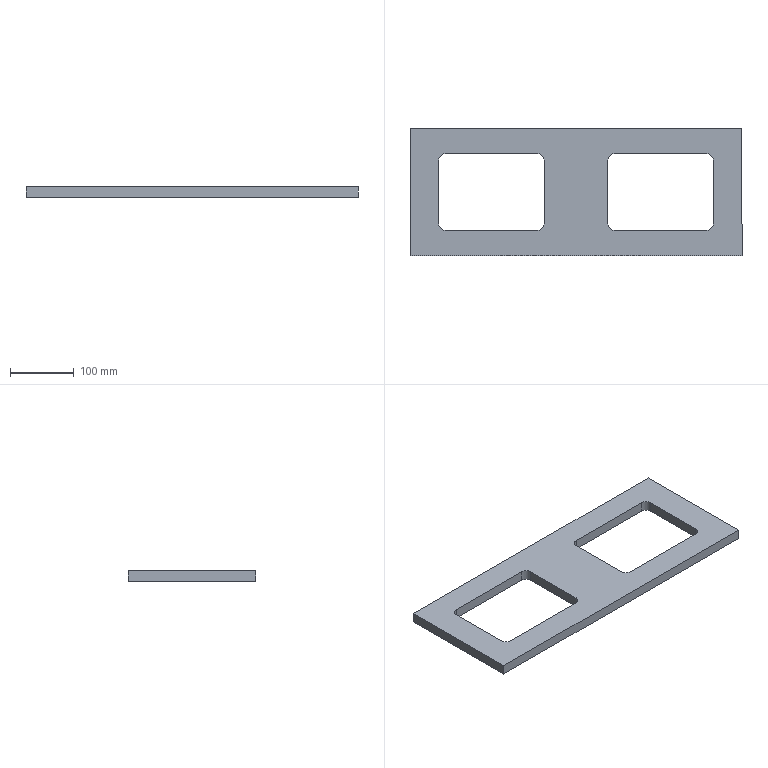Part | SolidWorks | features Extrusion 1 | 1 solid | 22 faces | box 520 x 200 x 16 mm | volume 1033147 mm3 | plane 14 | cylinder 8 | commonest cylinder face diameters 20 x8
STEP:
#1=CARTESIAN_POINT('',(-50.151,129.965,16.));
#2=VERTEX_POINT('',#1);
#3=CARTESIAN_POINT('',(-60.151,119.965,16.));
#4=VERTEX_POINT('',#3);
#5=CARTESIAN_POINT('',(-50.151,119.965,16.));
#6=DIRECTION('',(0.,0.,1.));
#7=DIRECTION('',(-1.,0.,0.));
#8=AXIS2_PLACEMENT_3D('',#5,#6,#7);
#9=CIRCLE('',#8,10.);
#10=EDGE_CURVE('',#2,#4,#9,.T.);
#11=ORIENTED_EDGE('',*,*,#10,.F.);
#12=CARTESIAN_POINT('',(94.849,129.965,16.));
#13=VERTEX_POINT('',#12);
#14=CARTESIAN_POINT('',(94.849,129.965,16.));
#15=DIRECTION('',(-1.,0.,0.));
#16=VECTOR('',#15,1000.);
#17=LINE('',#14,#16);
#18=EDGE_CURVE('',#13,#2,#17,.T.);
#19=ORIENTED_EDGE('',*,*,#18,.F.);
#20=CARTESIAN_POINT('',(104.849,119.965,16.));
#21=VERTEX_POINT('',#20);
#22=CARTESIAN_POINT('',(94.849,119.965,16.));
#23=DIRECTION('',(0.,0.,1.));
#24=DIRECTION('',(-1.,0.,0.));
#25=AXIS2_PLACEMENT_3D('',#22,#23,#24);
#26=CIRCLE('',#25,10.);
#27=EDGE_CURVE('',#21,#13,#26,.T.);
#28=ORIENTED_EDGE('',*,*,#27,.F.);
#29=CARTESIAN_POINT('',(104.849,19.965,16.));
#30=VERTEX_POINT('',#29);
#31=CARTESIAN_POINT('',(104.849,19.965,16.));
#32=DIRECTION('',(0.,1.,0.));
#33=VECTOR('',#32,1000.);
#34=LINE('',#31,#33);
#35=EDGE_CURVE('',#30,#21,#34,.T.);
#36=ORIENTED_EDGE('',*,*,#35,.F.);
#37=CARTESIAN_POINT('',(94.849,9.965,16.));
#38=VERTEX_POINT('',#37);
#39=CARTESIAN_POINT('',(94.849,19.965,16.));
#40=DIRECTION('',(0.,0.,1.));
#41=DIRECTION('',(1.,0.,0.));
#42=AXIS2_PLACEMENT_3D('',#39,#40,#41);
#43=CIRCLE('',#42,10.);
#44=EDGE_CURVE('',#38,#30,#43,.T.);
#45=ORIENTED_EDGE('',*,*,#44,.F.);
#46=CARTESIAN_POINT('',(-50.151,9.965,16.));
#47=VERTEX_POINT('',#46);
#48=CARTESIAN_POINT('',(-50.151,9.965,16.));
#49=DIRECTION('',(1.,0.,0.));
#50=VECTOR('',#49,1000.);
#51=LINE('',#48,#50);
#52=EDGE_CURVE('',#47,#38,#51,.T.);
#53=ORIENTED_EDGE('',*,*,#52,.F.);
#54=CARTESIAN_POINT('',(-60.151,19.965,16.));
#55=VERTEX_POINT('',#54);
#56=CARTESIAN_POINT('',(-50.151,19.965,16.));
#57=DIRECTION('',(0.,0.,1.));
#58=DIRECTION('',(-1.,0.,0.));
#59=AXIS2_PLACEMENT_3D('',#56,#57,#58);
#60=CIRCLE('',#59,10.);
#61=EDGE_CURVE('',#55,#47,#60,.T.);
#62=ORIENTED_EDGE('',*,*,#61,.F.);
#63=CARTESIAN_POINT('',(-60.151,119.965,16.));
#64=DIRECTION('',(0.,-1.,0.));
#65=VECTOR('',#64,1000.);
#66=LINE('',#63,#65);
#67=EDGE_CURVE('',#4,#55,#66,.T.);
#68=ORIENTED_EDGE('',*,*,#67,.F.);
#69=EDGE_LOOP('',(#11,#19,#28,#36,#45,#53,#62,#68));
#70=FACE_BOUND('',#69,.T.);
#71=CARTESIAN_POINT('',(-105.151,169.965,16.));
#72=VERTEX_POINT('',#71);
#73=CARTESIAN_POINT('',(-105.151,-30.035,16.));
#74=VERTEX_POINT('',#73);
#75=CARTESIAN_POINT('',(-105.151,-30.035,16.));
#76=DIRECTION('',(0.,-1.,0.));
#77=VECTOR('',#76,1000.);
#78=LINE('',#75,#77);
#79=EDGE_CURVE('',#72,#74,#78,.T.);
#80=ORIENTED_EDGE('',*,*,#79,.T.);
#81=CARTESIAN_POINT('',(414.849,-30.035,16.));
#82=VERTEX_POINT('',#81);
#83=CARTESIAN_POINT('',(414.849,-30.035,16.));
#84=DIRECTION('',(1.,0.,0.));
#85=VECTOR('',#84,1000.);
#86=LINE('',#83,#85);
#87=EDGE_CURVE('',#74,#82,#86,.T.);
#88=ORIENTED_EDGE('',*,*,#87,.T.);
#89=CARTESIAN_POINT('',(414.849,169.965,16.));
#90=VERTEX_POINT('',#89);
#91=CARTESIAN_POINT('',(414.849,169.965,16.));
#92=DIRECTION('',(0.,1.,0.));
#93=VECTOR('',#92,1000.);
#94=LINE('',#91,#93);
#95=EDGE_CURVE('',#82,#90,#94,.T.);
#96=ORIENTED_EDGE('',*,*,#95,.T.);
#97=CARTESIAN_POINT('',(-105.151,169.965,16.));
#98=DIRECTION('',(-1.,0.,0.));
#99=VECTOR('',#98,1000.);
#100=LINE('',#97,#99);
#101=EDGE_CURVE('',#90,#72,#100,.T.);
#102=ORIENTED_EDGE('',*,*,#101,.T.);
#103=EDGE_LOOP('',(#80,#88,#96,#102));
#104=FACE_OUTER_BOUND('',#103,.T.);
#105=CARTESIAN_POINT('',(359.849,9.965,16.));
#106=VERTEX_POINT('',#105);
#107=CARTESIAN_POINT('',(369.849,19.965,16.));
#108=VERTEX_POINT('',#107);
#109=CARTESIAN_POINT('',(359.849,19.965,16.));
#110=DIRECTION('',(0.,0.,1.));
#111=DIRECTION('',(1.,0.,0.));
#112=AXIS2_PLACEMENT_3D('',#109,#110,#111);
#113=CIRCLE('',#112,10.);
#114=EDGE_CURVE('',#106,#108,#113,.T.);
#115=ORIENTED_EDGE('',*,*,#114,.F.);
#116=CARTESIAN_POINT('',(214.849,9.965,16.));
#117=VERTEX_POINT('',#116);
#118=CARTESIAN_POINT('',(359.849,9.965,16.));
#119=DIRECTION('',(1.,0.,0.));
#120=VECTOR('',#119,1000.);
#121=LINE('',#118,#120);
#122=EDGE_CURVE('',#117,#106,#121,.T.);
#123=ORIENTED_EDGE('',*,*,#122,.F.);
#124=CARTESIAN_POINT('',(204.849,19.965,16.));
#125=VERTEX_POINT('',#124);
#126=CARTESIAN_POINT('',(214.849,19.965,16.));
#127=DIRECTION('',(0.,0.,1.));
#128=DIRECTION('',(-1.,0.,0.));
#129=AXIS2_PLACEMENT_3D('',#126,#127,#128);
#130=CIRCLE('',#129,10.);
#131=EDGE_CURVE('',#125,#117,#130,.T.);
#132=ORIENTED_EDGE('',*,*,#131,.F.);
#133=CARTESIAN_POINT('',(204.849,119.965,16.));
#134=VERTEX_POINT('',#133);
#135=CARTESIAN_POINT('',(204.849,19.965,16.));
#136=DIRECTION('',(0.,-1.,0.));
#137=VECTOR('',#136,1000.);
#138=LINE('',#135,#137);
#139=EDGE_CURVE('',#134,#125,#138,.T.);
#140=ORIENTED_EDGE('',*,*,#139,.F.);
#141=CARTESIAN_POINT('',(214.849,129.965,16.));
#142=VERTEX_POINT('',#141);
#143=CARTESIAN_POINT('',(214.849,119.965,16.));
#144=DIRECTION('',(0.,0.,1.));
#145=DIRECTION('',(1.,0.,0.));
#146=AXIS2_PLACEMENT_3D('',#143,#144,#145);
#147=CIRCLE('',#146,10.);
#148=EDGE_CURVE('',#142,#134,#147,.T.);
#149=ORIENTED_EDGE('',*,*,#148,.F.);
#150=CARTESIAN_POINT('',(359.849,129.965,16.));
#151=VERTEX_POINT('',#150);
#152=CARTESIAN_POINT('',(214.849,129.965,16.));
#153=DIRECTION('',(-1.,0.,0.));
#154=VECTOR('',#153,1000.);
#155=LINE('',#152,#154);
#156=EDGE_CURVE('',#151,#142,#155,.T.);
#157=ORIENTED_EDGE('',*,*,#156,.F.);
#158=CARTESIAN_POINT('',(369.849,119.965,16.));
#159=VERTEX_POINT('',#158);
#160=CARTESIAN_POINT('',(359.849,119.965,16.));
#161=DIRECTION('',(0.,0.,1.));
#162=DIRECTION('',(1.,0.,0.));
#163=AXIS2_PLACEMENT_3D('',#160,#161,#162);
#164=CIRCLE('',#163,10.);
#165=EDGE_CURVE('',#159,#151,#164,.T.);
#166=ORIENTED_EDGE('',*,*,#165,.F.);
#167=CARTESIAN_POINT('',(369.849,119.965,16.));
#168=DIRECTION('',(0.,1.,0.));
#169=VECTOR('',#168,1000.);
#170=LINE('',#167,#169);
#171=EDGE_CURVE('',#108,#159,#170,.T.);
#172=ORIENTED_EDGE('',*,*,#171,.F.);
#173=EDGE_LOOP('',(#115,#123,#132,#140,#149,#157,#166,#172));
#174=FACE_BOUND('',#173,.T.);
#175=CARTESIAN_POINT('',(0.,0.,16.));
#176=DIRECTION('',(0.,0.,-1.));
#177=DIRECTION('',(-1.,0.,0.));
#178=AXIS2_PLACEMENT_3D('',#175,#176,#177);
#179=PLANE('',#178);
#180=ADVANCED_FACE('',(#70,#104,#174),#179,.F.);
#181=CARTESIAN_POINT('',(-105.151,169.965,0.));
#182=VERTEX_POINT('',#181);
#183=CARTESIAN_POINT('',(-105.151,-30.035,0.));
#184=VERTEX_POINT('',#183);
#185=CARTESIAN_POINT('',(-105.151,-30.035,0.));
#186=DIRECTION('',(0.,-1.,0.));
#187=VECTOR('',#186,1000.);
#188=LINE('',#185,#187);
#189=EDGE_CURVE('',#182,#184,#188,.T.);
#190=ORIENTED_EDGE('',*,*,#189,.F.);
#191=CARTESIAN_POINT('',(414.849,169.965,0.));
#192=VERTEX_POINT('',#191);
#193=CARTESIAN_POINT('',(-105.151,169.965,0.));
#194=DIRECTION('',(-1.,0.,0.));
#195=VECTOR('',#194,1000.);
#196=LINE('',#193,#195);
#197=EDGE_CURVE('',#192,#182,#196,.T.);
#198=ORIENTED_EDGE('',*,*,#197,.F.);
#199=CARTESIAN_POINT('',(414.849,-30.035,0.));
#200=VERTEX_POINT('',#199);
#201=CARTESIAN_POINT('',(414.849,169.965,0.));
#202=DIRECTION('',(0.,1.,0.));
#203=VECTOR('',#202,1000.);
#204=LINE('',#201,#203);
#205=EDGE_CURVE('',#200,#192,#204,.T.);
#206=ORIENTED_EDGE('',*,*,#205,.F.);
#207=CARTESIAN_POINT('',(414.849,-30.035,0.));
#208=DIRECTION('',(1.,0.,0.));
#209=VECTOR('',#208,1000.);
#210=LINE('',#207,#209);
#211=EDGE_CURVE('',#184,#200,#210,.T.);
#212=ORIENTED_EDGE('',*,*,#211,.F.);
#213=EDGE_LOOP('',(#190,#198,#206,#212));
#214=FACE_OUTER_BOUND('',#213,.T.);
#215=CARTESIAN_POINT('',(94.849,129.965,0.));
#216=VERTEX_POINT('',#215);
#217=CARTESIAN_POINT('',(-50.151,129.965,0.));
#218=VERTEX_POINT('',#217);
#219=CARTESIAN_POINT('',(94.849,129.965,0.));
#220=DIRECTION('',(-1.,0.,0.));
#221=VECTOR('',#220,1000.);
#222=LINE('',#219,#221);
#223=EDGE_CURVE('',#216,#218,#222,.T.);
#224=ORIENTED_EDGE('',*,*,#223,.T.);
#225=CARTESIAN_POINT('',(-60.151,119.965,0.));
#226=VERTEX_POINT('',#225);
#227=CARTESIAN_POINT('',(-50.151,119.965,0.));
#228=DIRECTION('',(0.,0.,1.));
#229=DIRECTION('',(-1.,0.,0.));
#230=AXIS2_PLACEMENT_3D('',#227,#228,#229);
#231=CIRCLE('',#230,10.);
#232=EDGE_CURVE('',#218,#226,#231,.T.);
#233=ORIENTED_EDGE('',*,*,#232,.T.);
#234=CARTESIAN_POINT('',(-60.151,19.965,0.));
#235=VERTEX_POINT('',#234);
#236=CARTESIAN_POINT('',(-60.151,119.965,0.));
#237=DIRECTION('',(0.,-1.,0.));
#238=VECTOR('',#237,1000.);
#239=LINE('',#236,#238);
#240=EDGE_CURVE('',#226,#235,#239,.T.);
#241=ORIENTED_EDGE('',*,*,#240,.T.);
#242=CARTESIAN_POINT('',(-50.151,9.965,0.));
#243=VERTEX_POINT('',#242);
#244=CARTESIAN_POINT('',(-50.151,19.965,0.));
#245=DIRECTION('',(0.,0.,1.));
#246=DIRECTION('',(-1.,0.,0.));
#247=AXIS2_PLACEMENT_3D('',#244,#245,#246);
#248=CIRCLE('',#247,10.);
#249=EDGE_CURVE('',#235,#243,#248,.T.);
#250=ORIENTED_EDGE('',*,*,#249,.T.);
#251=CARTESIAN_POINT('',(94.849,9.965,0.));
#252=VERTEX_POINT('',#251);
#253=CARTESIAN_POINT('',(-35.652,9.965,0.));
#254=DIRECTION('',(1.,0.,0.));
#255=VECTOR('',#254,1000.);
#256=LINE('',#253,#255);
#257=EDGE_CURVE('',#243,#252,#256,.T.);
#258=ORIENTED_EDGE('',*,*,#257,.T.);
#259=CARTESIAN_POINT('',(104.849,19.965,0.));
#260=VERTEX_POINT('',#259);
#261=CARTESIAN_POINT('',(94.849,19.965,0.));
#262=DIRECTION('',(0.,0.,1.));
#263=DIRECTION('',(1.,0.,0.));
#264=AXIS2_PLACEMENT_3D('',#261,#262,#263);
#265=CIRCLE('',#264,10.);
#266=EDGE_CURVE('',#252,#260,#265,.T.);
#267=ORIENTED_EDGE('',*,*,#266,.T.);
#268=CARTESIAN_POINT('',(104.849,119.965,0.));
#269=VERTEX_POINT('',#268);
#270=CARTESIAN_POINT('',(104.849,19.965,0.));
#271=DIRECTION('',(0.,1.,0.));
#272=VECTOR('',#271,1000.);
#273=LINE('',#270,#272);
#274=EDGE_CURVE('',#260,#269,#273,.T.);
#275=ORIENTED_EDGE('',*,*,#274,.T.);
#276=CARTESIAN_POINT('',(94.849,119.965,0.));
#277=DIRECTION('',(0.,0.,1.));
#278=DIRECTION('',(-1.,0.,0.));
#279=AXIS2_PLACEMENT_3D('',#276,#277,#278);
#280=CIRCLE('',#279,10.);
#281=EDGE_CURVE('',#269,#216,#280,.T.);
#282=ORIENTED_EDGE('',*,*,#281,.T.);
#283=EDGE_LOOP('',(#224,#233,#241,#250,#258,#267,#275,#282));
#284=FACE_BOUND('',#283,.T.);
#285=CARTESIAN_POINT('',(214.849,9.965,0.));
#286=VERTEX_POINT('',#285);
#287=CARTESIAN_POINT('',(359.849,9.965,0.));
#288=VERTEX_POINT('',#287);
#289=CARTESIAN_POINT('',(345.35,9.965,0.));
#290=DIRECTION('',(1.,0.,0.));
#291=VECTOR('',#290,1000.);
#292=LINE('',#289,#291);
#293=EDGE_CURVE('',#286,#288,#292,.T.);
#294=ORIENTED_EDGE('',*,*,#293,.T.);
#295=CARTESIAN_POINT('',(369.849,19.965,0.));
#296=VERTEX_POINT('',#295);
#297=CARTESIAN_POINT('',(359.849,19.965,0.));
#298=DIRECTION('',(0.,0.,1.));
#299=DIRECTION('',(1.,0.,0.));
#300=AXIS2_PLACEMENT_3D('',#297,#298,#299);
#301=CIRCLE('',#300,10.);
#302=EDGE_CURVE('',#288,#296,#301,.T.);
#303=ORIENTED_EDGE('',*,*,#302,.T.);
#304=CARTESIAN_POINT('',(369.849,119.965,0.));
#305=VERTEX_POINT('',#304);
#306=CARTESIAN_POINT('',(369.849,119.965,0.));
#307=DIRECTION('',(0.,1.,0.));
#308=VECTOR('',#307,1000.);
#309=LINE('',#306,#308);
#310=EDGE_CURVE('',#296,#305,#309,.T.);
#311=ORIENTED_EDGE('',*,*,#310,.T.);
#312=CARTESIAN_POINT('',(359.849,129.965,0.));
#313=VERTEX_POINT('',#312);
#314=CARTESIAN_POINT('',(359.849,119.965,0.));
#315=DIRECTION('',(0.,0.,1.));
#316=DIRECTION('',(1.,0.,0.));
#317=AXIS2_PLACEMENT_3D('',#314,#315,#316);
#318=CIRCLE('',#317,10.);
#319=EDGE_CURVE('',#305,#313,#318,.T.);
#320=ORIENTED_EDGE('',*,*,#319,.T.);
#321=CARTESIAN_POINT('',(214.849,129.965,0.));
#322=VERTEX_POINT('',#321);
#323=CARTESIAN_POINT('',(214.849,129.965,0.));
#324=DIRECTION('',(-1.,0.,0.));
#325=VECTOR('',#324,1000.);
#326=LINE('',#323,#325);
#327=EDGE_CURVE('',#313,#322,#326,.T.);
#328=ORIENTED_EDGE('',*,*,#327,.T.);
#329=CARTESIAN_POINT('',(204.849,119.965,0.));
#330=VERTEX_POINT('',#329);
#331=CARTESIAN_POINT('',(214.849,119.965,0.));
#332=DIRECTION('',(0.,0.,1.));
#333=DIRECTION('',(1.,0.,0.));
#334=AXIS2_PLACEMENT_3D('',#331,#332,#333);
#335=CIRCLE('',#334,10.);
#336=EDGE_CURVE('',#322,#330,#335,.T.);
#337=ORIENTED_EDGE('',*,*,#336,.T.);
#338=CARTESIAN_POINT('',(204.849,19.965,0.));
#339=VERTEX_POINT('',#338);
#340=CARTESIAN_POINT('',(204.849,19.965,0.));
#341=DIRECTION('',(0.,-1.,0.));
#342=VECTOR('',#341,1000.);
#343=LINE('',#340,#342);
#344=EDGE_CURVE('',#330,#339,#343,.T.);
#345=ORIENTED_EDGE('',*,*,#344,.T.);
#346=CARTESIAN_POINT('',(214.849,19.965,0.));
#347=DIRECTION('',(0.,0.,1.));
#348=DIRECTION('',(-1.,0.,0.));
#349=AXIS2_PLACEMENT_3D('',#346,#347,#348);
#350=CIRCLE('',#349,10.);
#351=EDGE_CURVE('',#339,#286,#350,.T.);
#352=ORIENTED_EDGE('',*,*,#351,.T.);
#353=EDGE_LOOP('',(#294,#303,#311,#320,#328,#337,#345,#352));
#354=FACE_BOUND('',#353,.T.);
#355=CARTESIAN_POINT('',(0.,0.,0.));
#356=DIRECTION('',(0.,0.,-1.));
#357=DIRECTION('',(-1.,0.,0.));
#358=AXIS2_PLACEMENT_3D('',#355,#356,#357);
#359=PLANE('',#358);
#360=ADVANCED_FACE('',(#214,#284,#354),#359,.T.);
#361=ORIENTED_EDGE('',*,*,#189,.T.);
#362=CARTESIAN_POINT('',(-105.151,-30.035,16.));
#363=DIRECTION('',(0.,0.,-1.));
#364=VECTOR('',#363,1000.);
#365=LINE('',#362,#364);
#366=EDGE_CURVE('',#74,#184,#365,.T.);
#367=ORIENTED_EDGE('',*,*,#366,.F.);
#368=ORIENTED_EDGE('',*,*,#79,.F.);
#369=CARTESIAN_POINT('',(-105.151,169.965,16.));
#370=DIRECTION('',(0.,0.,-1.));
#371=VECTOR('',#370,1000.);
#372=LINE('',#369,#371);
#373=EDGE_CURVE('',#72,#182,#372,.T.);
#374=ORIENTED_EDGE('',*,*,#373,.T.);
#375=EDGE_LOOP('',(#361,#367,#368,#374));
#376=FACE_OUTER_BOUND('',#375,.T.);
#377=CARTESIAN_POINT('',(-105.151,-30.035,16.));
#378=DIRECTION('',(1.,0.,0.));
#379=DIRECTION('',(0.,0.,-1.));
#380=AXIS2_PLACEMENT_3D('',#377,#378,#379);
#381=PLANE('',#380);
#382=ADVANCED_FACE('',(#376),#381,.F.);
#383=ORIENTED_EDGE('',*,*,#211,.T.);
#384=CARTESIAN_POINT('',(414.849,-30.035,16.));
#385=DIRECTION('',(0.,0.,-1.));
#386=VECTOR('',#385,1000.);
#387=LINE('',#384,#386);
#388=EDGE_CURVE('',#82,#200,#387,.T.);
#389=ORIENTED_EDGE('',*,*,#388,.F.);
#390=ORIENTED_EDGE('',*,*,#87,.F.);
#391=ORIENTED_EDGE('',*,*,#366,.T.);
#392=EDGE_LOOP('',(#383,#389,#390,#391));
#393=FACE_OUTER_BOUND('',#392,.T.);
#394=CARTESIAN_POINT('',(414.849,-30.035,16.));
#395=DIRECTION('',(0.,1.,0.));
#396=DIRECTION('',(-1.,0.,0.));
#397=AXIS2_PLACEMENT_3D('',#394,#395,#396);
#398=PLANE('',#397);
#399=ADVANCED_FACE('',(#393),#398,.F.);
#400=ORIENTED_EDGE('',*,*,#205,.T.);
#401=CARTESIAN_POINT('',(414.849,169.965,16.));
#402=DIRECTION('',(0.,0.,-1.));
#403=VECTOR('',#402,1000.);
#404=LINE('',#401,#403);
#405=EDGE_CURVE('',#90,#192,#404,.T.);
#406=ORIENTED_EDGE('',*,*,#405,.F.);
#407=ORIENTED_EDGE('',*,*,#95,.F.);
#408=ORIENTED_EDGE('',*,*,#388,.T.);
#409=EDGE_LOOP('',(#400,#406,#407,#408));
#410=FACE_OUTER_BOUND('',#409,.T.);
#411=CARTESIAN_POINT('',(414.849,169.965,16.));
#412=DIRECTION('',(-1.,0.,0.));
#413=DIRECTION('',(0.,-1.,0.));
#414=AXIS2_PLACEMENT_3D('',#411,#412,#413);
#415=PLANE('',#414);
#416=ADVANCED_FACE('',(#410),#415,.F.);
#417=ORIENTED_EDGE('',*,*,#197,.T.);
#418=ORIENTED_EDGE('',*,*,#373,.F.);
#419=ORIENTED_EDGE('',*,*,#101,.F.);
#420=ORIENTED_EDGE('',*,*,#405,.T.);
#421=EDGE_LOOP('',(#417,#418,#419,#420));
#422=FACE_OUTER_BOUND('',#421,.T.);
#423=CARTESIAN_POINT('',(-105.151,169.965,16.));
#424=DIRECTION('',(0.,-1.,0.));
#425=DIRECTION('',(0.,0.,-1.));
#426=AXIS2_PLACEMENT_3D('',#423,#424,#425);
#427=PLANE('',#426);
#428=ADVANCED_FACE('',(#422),#427,.F.);
#429=ORIENTED_EDGE('',*,*,#232,.F.);
#430=CARTESIAN_POINT('',(-50.151,129.965,16.));
#431=DIRECTION('',(0.,0.,-1.));
#432=VECTOR('',#431,1000.);
#433=LINE('',#430,#432);
#434=EDGE_CURVE('',#2,#218,#433,.T.);
#435=ORIENTED_EDGE('',*,*,#434,.F.);
#436=ORIENTED_EDGE('',*,*,#10,.T.);
#437=CARTESIAN_POINT('',(-60.151,119.965,16.));
#438=DIRECTION('',(0.,0.,-1.));
#439=VECTOR('',#438,1000.);
#440=LINE('',#437,#439);
#441=EDGE_CURVE('',#4,#226,#440,.T.);
#442=ORIENTED_EDGE('',*,*,#441,.T.);
#443=EDGE_LOOP('',(#429,#435,#436,#442));
#444=FACE_OUTER_BOUND('',#443,.T.);
#445=CARTESIAN_POINT('',(-50.151,119.965,16.));
#446=DIRECTION('',(0.,0.,-1.));
#447=DIRECTION('',(-1.,0.,0.));
#448=AXIS2_PLACEMENT_3D('',#445,#446,#447);
#449=CYLINDRICAL_SURFACE('',#448,10.);
#450=ADVANCED_FACE('',(#444),#449,.F.);
#451=ORIENTED_EDGE('',*,*,#240,.F.);
#452=ORIENTED_EDGE('',*,*,#441,.F.);
#453=ORIENTED_EDGE('',*,*,#67,.T.);
#454=CARTESIAN_POINT('',(-60.151,19.965,16.));
#455=DIRECTION('',(0.,0.,-1.));
#456=VECTOR('',#455,1000.);
#457=LINE('',#454,#456);
#458=EDGE_CURVE('',#55,#235,#457,.T.);
#459=ORIENTED_EDGE('',*,*,#458,.T.);
#460=EDGE_LOOP('',(#451,#452,#453,#459));
#461=FACE_OUTER_BOUND('',#460,.T.);
#462=CARTESIAN_POINT('',(-60.151,119.965,16.));
#463=DIRECTION('',(1.,0.,0.));
#464=DIRECTION('',(0.,0.,-1.));
#465=AXIS2_PLACEMENT_3D('',#462,#463,#464);
#466=PLANE('',#465);
#467=ADVANCED_FACE('',(#461),#466,.T.);
#468=ORIENTED_EDGE('',*,*,#249,.F.);
#469=ORIENTED_EDGE('',*,*,#458,.F.);
#470=ORIENTED_EDGE('',*,*,#61,.T.);
#471=CARTESIAN_POINT('',(-50.151,9.965,16.));
#472=DIRECTION('',(0.,0.,-1.));
#473=VECTOR('',#472,1000.);
#474=LINE('',#471,#473);
#475=EDGE_CURVE('',#47,#243,#474,.T.);
#476=ORIENTED_EDGE('',*,*,#475,.T.);
#477=EDGE_LOOP('',(#468,#469,#470,#476));
#478=FACE_OUTER_BOUND('',#477,.T.);
#479=CARTESIAN_POINT('',(-50.151,19.965,16.));
#480=DIRECTION('',(0.,0.,-1.));
#481=DIRECTION('',(-1.,0.,0.));
#482=AXIS2_PLACEMENT_3D('',#479,#480,#481);
#483=CYLINDRICAL_SURFACE('',#482,10.);
#484=ADVANCED_FACE('',(#478),#483,.F.);
#485=ORIENTED_EDGE('',*,*,#257,.F.);
#486=ORIENTED_EDGE('',*,*,#475,.F.);
#487=ORIENTED_EDGE('',*,*,#52,.T.);
#488=CARTESIAN_POINT('',(94.849,9.965,16.));
#489=DIRECTION('',(0.,0.,-1.));
#490=VECTOR('',#489,1000.);
#491=LINE('',#488,#490);
#492=EDGE_CURVE('',#38,#252,#491,.T.);
#493=ORIENTED_EDGE('',*,*,#492,.T.);
#494=EDGE_LOOP('',(#485,#486,#487,#493));
#495=FACE_OUTER_BOUND('',#494,.T.);
#496=CARTESIAN_POINT('',(-35.652,9.965,16.));
#497=DIRECTION('',(0.,1.,0.));
#498=DIRECTION('',(0.,0.,1.));
#499=AXIS2_PLACEMENT_3D('',#496,#497,#498);
#500=PLANE('',#499);
#501=ADVANCED_FACE('',(#495),#500,.T.);
#502=ORIENTED_EDGE('',*,*,#266,.F.);
#503=ORIENTED_EDGE('',*,*,#492,.F.);
#504=ORIENTED_EDGE('',*,*,#44,.T.);
#505=CARTESIAN_POINT('',(104.849,19.965,16.));
#506=DIRECTION('',(0.,0.,-1.));
#507=VECTOR('',#506,1000.);
#508=LINE('',#505,#507);
#509=EDGE_CURVE('',#30,#260,#508,.T.);
#510=ORIENTED_EDGE('',*,*,#509,.T.);
#511=EDGE_LOOP('',(#502,#503,#504,#510));
#512=FACE_OUTER_BOUND('',#511,.T.);
#513=CARTESIAN_POINT('',(94.849,19.965,16.));
#514=DIRECTION('',(0.,0.,-1.));
#515=DIRECTION('',(-1.,0.,0.));
#516=AXIS2_PLACEMENT_3D('',#513,#514,#515);
#517=CYLINDRICAL_SURFACE('',#516,10.);
#518=ADVANCED_FACE('',(#512),#517,.F.);
#519=ORIENTED_EDGE('',*,*,#274,.F.);
#520=ORIENTED_EDGE('',*,*,#509,.F.);
#521=ORIENTED_EDGE('',*,*,#35,.T.);
#522=CARTESIAN_POINT('',(104.849,119.965,16.));
#523=DIRECTION('',(0.,0.,-1.));
#524=VECTOR('',#523,1000.);
#525=LINE('',#522,#524);
#526=EDGE_CURVE('',#21,#269,#525,.T.);
#527=ORIENTED_EDGE('',*,*,#526,.T.);
#528=EDGE_LOOP('',(#519,#520,#521,#527));
#529=FACE_OUTER_BOUND('',#528,.T.);
#530=CARTESIAN_POINT('',(104.849,19.965,16.));
#531=DIRECTION('',(-1.,0.,0.));
#532=DIRECTION('',(0.,0.,1.));
#533=AXIS2_PLACEMENT_3D('',#530,#531,#532);
#534=PLANE('',#533);
#535=ADVANCED_FACE('',(#529),#534,.T.);
#536=ORIENTED_EDGE('',*,*,#281,.F.);
#537=ORIENTED_EDGE('',*,*,#526,.F.);
#538=ORIENTED_EDGE('',*,*,#27,.T.);
#539=CARTESIAN_POINT('',(94.849,129.965,16.));
#540=DIRECTION('',(0.,0.,-1.));
#541=VECTOR('',#540,1000.);
#542=LINE('',#539,#541);
#543=EDGE_CURVE('',#13,#216,#542,.T.);
#544=ORIENTED_EDGE('',*,*,#543,.T.);
#545=EDGE_LOOP('',(#536,#537,#538,#544));
#546=FACE_OUTER_BOUND('',#545,.T.);
#547=CARTESIAN_POINT('',(94.849,119.965,16.));
#548=DIRECTION('',(0.,0.,-1.));
#549=DIRECTION('',(-1.,0.,0.));
#550=AXIS2_PLACEMENT_3D('',#547,#548,#549);
#551=CYLINDRICAL_SURFACE('',#550,10.);
#552=ADVANCED_FACE('',(#546),#551,.F.);
#553=ORIENTED_EDGE('',*,*,#223,.F.);
#554=ORIENTED_EDGE('',*,*,#543,.F.);
#555=ORIENTED_EDGE('',*,*,#18,.T.);
#556=ORIENTED_EDGE('',*,*,#434,.T.);
#557=EDGE_LOOP('',(#553,#554,#555,#556));
#558=FACE_OUTER_BOUND('',#557,.T.);
#559=CARTESIAN_POINT('',(94.849,129.965,16.));
#560=DIRECTION('',(0.,-1.,0.));
#561=DIRECTION('',(0.,0.,-1.));
#562=AXIS2_PLACEMENT_3D('',#559,#560,#561);
#563=PLANE('',#562);
#564=ADVANCED_FACE('',(#558),#563,.T.);
#565=ORIENTED_EDGE('',*,*,#302,.F.);
#566=CARTESIAN_POINT('',(359.849,9.965,16.));
#567=DIRECTION('',(0.,0.,-1.));
#568=VECTOR('',#567,1000.);
#569=LINE('',#566,#568);
#570=EDGE_CURVE('',#106,#288,#569,.T.);
#571=ORIENTED_EDGE('',*,*,#570,.F.);
#572=ORIENTED_EDGE('',*,*,#114,.T.);
#573=CARTESIAN_POINT('',(369.849,19.965,16.));
#574=DIRECTION('',(0.,0.,-1.));
#575=VECTOR('',#574,1000.);
#576=LINE('',#573,#575);
#577=EDGE_CURVE('',#108,#296,#576,.T.);
#578=ORIENTED_EDGE('',*,*,#577,.T.);
#579=EDGE_LOOP('',(#565,#571,#572,#578));
#580=FACE_OUTER_BOUND('',#579,.T.);
#581=CARTESIAN_POINT('',(359.849,19.965,16.));
#582=DIRECTION('',(0.,0.,-1.));
#583=DIRECTION('',(-1.,0.,0.));
#584=AXIS2_PLACEMENT_3D('',#581,#582,#583);
#585=CYLINDRICAL_SURFACE('',#584,10.);
#586=ADVANCED_FACE('',(#580),#585,.F.);
#587=ORIENTED_EDGE('',*,*,#310,.F.);
#588=ORIENTED_EDGE('',*,*,#577,.F.);
#589=ORIENTED_EDGE('',*,*,#171,.T.);
#590=CARTESIAN_POINT('',(369.849,119.965,16.));
#591=DIRECTION('',(0.,0.,-1.));
#592=VECTOR('',#591,1000.);
#593=LINE('',#590,#592);
#594=EDGE_CURVE('',#159,#305,#593,.T.);
#595=ORIENTED_EDGE('',*,*,#594,.T.);
#596=EDGE_LOOP('',(#587,#588,#589,#595));
#597=FACE_OUTER_BOUND('',#596,.T.);
#598=CARTESIAN_POINT('',(369.849,119.965,16.));
#599=DIRECTION('',(-1.,0.,0.));
#600=DIRECTION('',(0.,0.,1.));
#601=AXIS2_PLACEMENT_3D('',#598,#599,#600);
#602=PLANE('',#601);
#603=ADVANCED_FACE('',(#597),#602,.T.);
#604=ORIENTED_EDGE('',*,*,#319,.F.);
#605=ORIENTED_EDGE('',*,*,#594,.F.);
#606=ORIENTED_EDGE('',*,*,#165,.T.);
#607=CARTESIAN_POINT('',(359.849,129.965,16.));
#608=DIRECTION('',(0.,0.,-1.));
#609=VECTOR('',#608,1000.);
#610=LINE('',#607,#609);
#611=EDGE_CURVE('',#151,#313,#610,.T.);
#612=ORIENTED_EDGE('',*,*,#611,.T.);
#613=EDGE_LOOP('',(#604,#605,#606,#612));
#614=FACE_OUTER_BOUND('',#613,.T.);
#615=CARTESIAN_POINT('',(359.849,119.965,16.));
#616=DIRECTION('',(0.,0.,-1.));
#617=DIRECTION('',(-1.,0.,0.));
#618=AXIS2_PLACEMENT_3D('',#615,#616,#617);
#619=CYLINDRICAL_SURFACE('',#618,10.);
#620=ADVANCED_FACE('',(#614),#619,.F.);
#621=ORIENTED_EDGE('',*,*,#327,.F.);
#622=ORIENTED_EDGE('',*,*,#611,.F.);
#623=ORIENTED_EDGE('',*,*,#156,.T.);
#624=CARTESIAN_POINT('',(214.849,129.965,16.));
#625=DIRECTION('',(0.,0.,-1.));
#626=VECTOR('',#625,1000.);
#627=LINE('',#624,#626);
#628=EDGE_CURVE('',#142,#322,#627,.T.);
#629=ORIENTED_EDGE('',*,*,#628,.T.);
#630=EDGE_LOOP('',(#621,#622,#623,#629));
#631=FACE_OUTER_BOUND('',#630,.T.);
#632=CARTESIAN_POINT('',(214.849,129.965,16.));
#633=DIRECTION('',(0.,-1.,0.));
#634=DIRECTION('',(0.,0.,-1.));
#635=AXIS2_PLACEMENT_3D('',#632,#633,#634);
#636=PLANE('',#635);
#637=ADVANCED_FACE('',(#631),#636,.T.);
#638=ORIENTED_EDGE('',*,*,#336,.F.);
#639=ORIENTED_EDGE('',*,*,#628,.F.);
#640=ORIENTED_EDGE('',*,*,#148,.T.);
#641=CARTESIAN_POINT('',(204.849,119.965,16.));
#642=DIRECTION('',(0.,0.,-1.));
#643=VECTOR('',#642,1000.);
#644=LINE('',#641,#643);
#645=EDGE_CURVE('',#134,#330,#644,.T.);
#646=ORIENTED_EDGE('',*,*,#645,.T.);
#647=EDGE_LOOP('',(#638,#639,#640,#646));
#648=FACE_OUTER_BOUND('',#647,.T.);
#649=CARTESIAN_POINT('',(214.849,119.965,16.));
#650=DIRECTION('',(0.,0.,-1.));
#651=DIRECTION('',(-1.,0.,0.));
#652=AXIS2_PLACEMENT_3D('',#649,#650,#651);
#653=CYLINDRICAL_SURFACE('',#652,10.);
#654=ADVANCED_FACE('',(#648),#653,.F.);
#655=ORIENTED_EDGE('',*,*,#344,.F.);
#656=ORIENTED_EDGE('',*,*,#645,.F.);
#657=ORIENTED_EDGE('',*,*,#139,.T.);
#658=CARTESIAN_POINT('',(204.849,19.965,16.));
#659=DIRECTION('',(0.,0.,-1.));
#660=VECTOR('',#659,1000.);
#661=LINE('',#658,#660);
#662=EDGE_CURVE('',#125,#339,#661,.T.);
#663=ORIENTED_EDGE('',*,*,#662,.T.);
#664=EDGE_LOOP('',(#655,#656,#657,#663));
#665=FACE_OUTER_BOUND('',#664,.T.);
#666=CARTESIAN_POINT('',(204.849,19.965,16.));
#667=DIRECTION('',(1.,0.,0.));
#668=DIRECTION('',(0.,0.,-1.));
#669=AXIS2_PLACEMENT_3D('',#666,#667,#668);
#670=PLANE('',#669);
#671=ADVANCED_FACE('',(#665),#670,.T.);
#672=ORIENTED_EDGE('',*,*,#351,.F.);
#673=ORIENTED_EDGE('',*,*,#662,.F.);
#674=ORIENTED_EDGE('',*,*,#131,.T.);
#675=CARTESIAN_POINT('',(214.849,9.965,16.));
#676=DIRECTION('',(0.,0.,-1.));
#677=VECTOR('',#676,1000.);
#678=LINE('',#675,#677);
#679=EDGE_CURVE('',#117,#286,#678,.T.);
#680=ORIENTED_EDGE('',*,*,#679,.T.);
#681=EDGE_LOOP('',(#672,#673,#674,#680));
#682=FACE_OUTER_BOUND('',#681,.T.);
#683=CARTESIAN_POINT('',(214.849,19.965,16.));
#684=DIRECTION('',(0.,0.,-1.));
#685=DIRECTION('',(-1.,0.,0.));
#686=AXIS2_PLACEMENT_3D('',#683,#684,#685);
#687=CYLINDRICAL_SURFACE('',#686,10.);
#688=ADVANCED_FACE('',(#682),#687,.F.);
#689=ORIENTED_EDGE('',*,*,#293,.F.);
#690=ORIENTED_EDGE('',*,*,#679,.F.);
#691=ORIENTED_EDGE('',*,*,#122,.T.);
#692=ORIENTED_EDGE('',*,*,#570,.T.);
#693=EDGE_LOOP('',(#689,#690,#691,#692));
#694=FACE_OUTER_BOUND('',#693,.T.);
#695=CARTESIAN_POINT('',(345.35,9.965,16.));
#696=DIRECTION('',(0.,1.,0.));
#697=DIRECTION('',(0.,0.,1.));
#698=AXIS2_PLACEMENT_3D('',#695,#696,#697);
#699=PLANE('',#698);
#700=ADVANCED_FACE('',(#694),#699,.T.);
#701=CLOSED_SHELL('',(#180,#360,#382,#399,#416,#428,#450,#467,#484,#501,#518,#535,#552,#564,#586,#603,#620,#637,#654,#671,#688,#700));
#702=MANIFOLD_SOLID_BREP('',#701);
#703=CARTESIAN_POINT('',(0.,0.,0.));
#704=DIRECTION('',(0.,0.,1.));
#705=DIRECTION('',(1.,0.,0.));
#706=AXIS2_PLACEMENT_3D('',#703,#704,#705);
#707=(LENGTH_UNIT()NAMED_UNIT(*)SI_UNIT(.MILLI.,.METRE.));
#708=UNCERTAINTY_MEASURE_WITH_UNIT(LENGTH_MEASURE(0.00001),#707,'','');
#709=(NAMED_UNIT(*)PLANE_ANGLE_UNIT()SI_UNIT($,.RADIAN.));
#710=(NAMED_UNIT(*)SI_UNIT($,.STERADIAN.)SOLID_ANGLE_UNIT());
#711=(GEOMETRIC_REPRESENTATION_CONTEXT(3)GLOBAL_UNCERTAINTY_ASSIGNED_CONTEXT((#708))GLOBAL_UNIT_ASSIGNED_CONTEXT((#707,#709,#710))REPRESENTATION_CONTEXT('',''));
#712=ADVANCED_BREP_SHAPE_REPRESENTATION('',(#702,#706),#711);